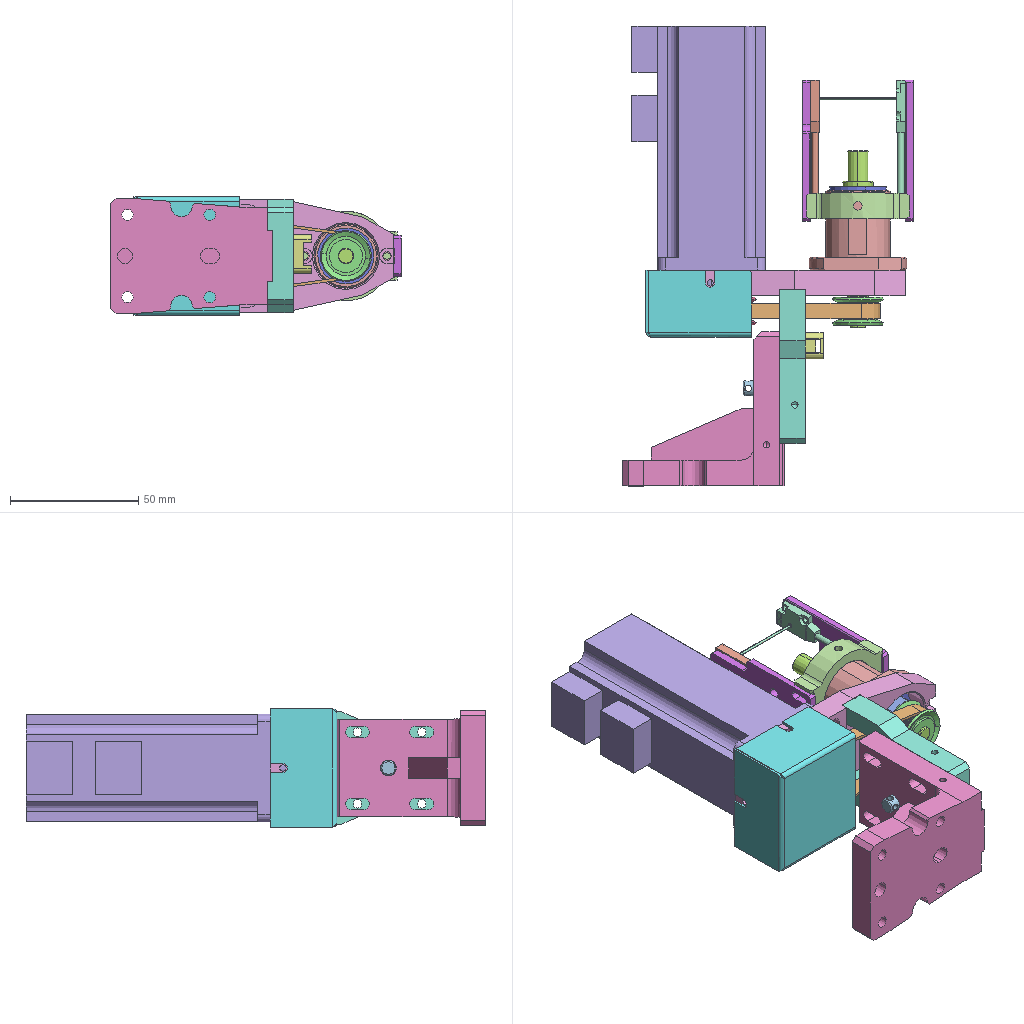Assembly | SolidWorks | 18 different items | 20 placed | box 113 x 179 x 46 mm
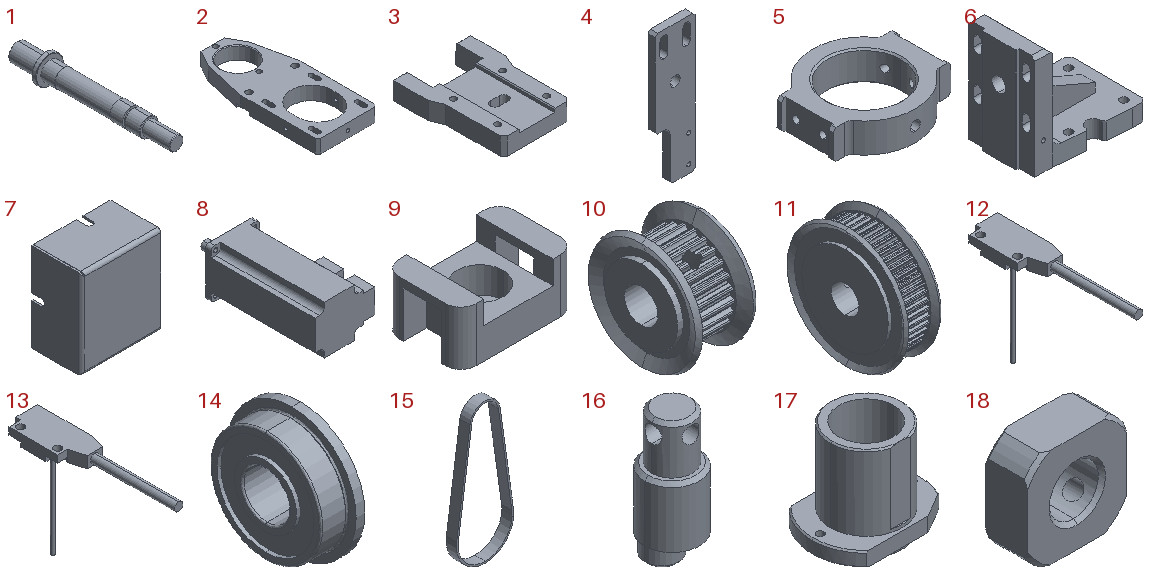Parts list (item | quantity | size | volume | features):
1 | x1 | 12 x 69 x 12 mm | 3193 mm3 | features ICE 3, Chamfer 1, Extrusion 1, RevCut 1
2 | x1 | 44 x 100 x 10 mm | 22505 mm3 | features ICE 7, HoleWzd 5, Chamfer 2, MirrorPattern 2, Cut 1, Extrusion 1, LPattern 1
3 | x1 | 44 x 60 x 10 mm | 17311 mm3 | features ICE 5, Chamfer 3, HoleWzd 3, Extrusion 1
4 | x2 | 16 x 3 x 55 mm | 2072 mm3 | features Chamfer 2, HoleWzd 2, Cut 1, Extrusion 1, Fillet 1, ICE 1
5 | x1 | 40 x 35 x 10 mm | 5332 mm3 | features ICE 3, Chamfer 2, HoleWzd 2, Extrusion 1, Fillet 1, MirrorPattern 1
6 | x1 | 62.8 x 45 x 60 mm | 46658 mm3 | features ICE 9, Chamfer 4, Cut 2, Extrusion 1, Fillet 1, HoleWzd 1, LPattern 1, MirrorPattern 1
7 | x1 | 41 x 26 x 46 mm | 4894 mm3 | features Chamfer 1, CornerFeat 1, Cut 1, EdgeFlange 1, FlatPattern 1, ICE 1, SMBaseFlange 1, SheetMetal 1
8 | x1 | 52 x 116 x 42 mm | 155076 mm3 | features ICE 7, Fillet 2, Extrusion 1
9 | x1 | 15 x 10 x 7 mm | 474.384 mm3 | features ICE 2, Extrusion 1, Fillet 1, HoleWzd 1
10 | x1 | 11 x 20 x 20 mm | 1710 mm3 | features BaseBody 1, CirPattern 1, HoleWzd 1, ICE 1
11 | x1 | 11 x 35 x 35 mm | 7284 mm3 | features BaseBody 3, CirPattern 1, HoleWzd 1
12 | x1 | 10 x 45.5 x 33.5 mm | 726.533 mm3 | features ICE 3, BaseBody 2
13 | x1 | 10 x 45.5 x 33.5 mm | 726.533 mm3 | features ICE 3, BaseBody 2
14 | x2 | 6 x 22 x 22 mm | 1366 mm3 | features BaseBody 1
15 | x1 | 33.828 x 6 x 82.868 mm | 1159 mm3 | features Extrusion 1
16 | x1 | 8 x 8 x 19.8 mm | 664.548 mm3 | features ICE 4, Chamfer 1, CirPattern 1, Extrusion 1
17 | x1 | 38 x 27 x 33 mm | 8754 mm3 | features ICE 5, Chamfer 1, Cut 1, Extrusion 1, HoleWzd 1, MirrorPattern 1
18 | x1 | 14 x 6.5 x 14 mm | 883.515 mm3 | features Chamfer 2, HoleWzd 2, ICE 2, CirPattern 1, Extrusion 1
Mates (type | each side: item.copy, entity, surface, feature):
Coincident | 3.1 face plane Boss-Extrude1 | 2.1 face plane Cut-Extrude13
Coincident | 3.1 face plane Boss-Extrude1 | 2.1 face plane Boss-Extrude1
Concentric | 1.1 face cylinder Boss-Extrude1 | 18.1 face cylinder M8x1.0 Tapped Hole1
Coincident | 2.1 face plane Boss-Extrude1 | 17.1 face plane Boss-Extrude2
Parallel | 2.1 face plane Boss-Extrude1 | 17.1 face plane Cut-Extrude1
Coincident | 2.1 face plane Boss-Extrude1 | 8.1 face plane Boss-Extrude1
Concentric | 1.1 face cylinder Boss-Extrude3 | 10.1 face cylinder Input 1
Coincident | 1.1 face plane Boss-Extrude1 | 10.1 face plane Input 1
Coincident | 10.1 face plane Input 1 | 11.1 face plane Input 1
Concentric | 8.1 face cylinder Boss-Extrude3 | 11.1 face cylinder Input 1
Concentric | 2.1 face cylinder Cut-Extrude1 | 17.1 face cylinder Boss-Extrude3
Concentric | 1.1 face cylinder Cut-Revolve1 | 17.1 face cylinder Boss-Extrude1
Concentric | 1.1 face cylinder Boss-Extrude1 | 18.1 face cylinder Boss-Extrude3
Concentric | 2.1 select_type:24 | 8.1 face cylinder Boss-Extrude3
Concentric | 15.1 face cylinder Boss-Extrude1 | 10.1 face cylinder Input 1
Concentric | 15.1 face cylinder Boss-Extrude1 | 11.1 face cylinder Input 1
DistanceDim | 11.1 face plane Input 1 | 15.1 face plane Boss-Extrude1
Parallel | 17.1 face plane Cut-Extrude1 | 2.1 face plane Boss-Extrude1
Parallel | 2.1 face plane Boss-Extrude1 | 8.1 face plane Boss-Extrude1
Coincident | 2.1 face plane Cut-Extrude13 | 3.1 face plane Boss-Extrude1
Width | 4.1 face plane Boss-Extrude1 | 4.1 face plane Boss-Extrude1 | 2.1 face plane Boss-Extrude1 | 2.1 face plane Boss-Extrude1
Coincident | 4.1 face plane Boss-Extrude1 | 4.2 face plane Boss-Extrude1
Concentric | 12.1 face cylinder Boss-Extrude1 | 13.1 face cylinder Boss-Extrude1
Coincident | 4.1 face plane Boss-Extrude1 | 12.1 face plane EX-11AD-1-solid1 | 2 times
DistanceDim | 12.1 face plane EX-11AD-1-solid1 | 4.1 face plane Boss-Extrude1
Coincident | 4.2 face plane Boss-Extrude1 | 13.1 face plane EX-11AD-1-solid1
Concentric | 4.2 face cylinder M2 Tapped Hole1 | 13.1 face cylinder EX-11AD-1-solid1
Concentric | 6.1 face cylinder Cut-Extrude9 | 16.1 face cylinder Boss-Extrude1
Coincident | 6.1 edge | 16.1 face plane Boss-Extrude1
Coincident | 1.1 face plane Boss-Extrude2 | 14.1 face plane Input 1
Coincident | 17.1 face plane Boss-Extrude1 | 14.1 face plane Input 1
Concentric | 17.1 face cylinder Boss-Extrude1 | 14.1 face cylinder Input 1
Coincident | 17.1 face plane Boss-Extrude3 | 14.2 face plane Input 1
Coincident | 18.1 face plane Boss-Extrude1 | 14.2 face plane Input 1
Concentric | 17.1 face cylinder Cut-Extrude2 | 14.2 face cylinder Input 1
Concentric | 17.1 face cylinder Boss-Extrude1 | 5.1 face cylinder Cut-Extrude1
Coincident | 4.1 face plane Boss-Extrude1 | 5.1 face plane Cut-Extrude2 | 2 times
Coincident | 4.2 face plane Boss-Extrude1 | 5.1 face plane Cut-Extrude2
DistanceDim | 4.1 face plane Boss-Extrude1 | 5.1 face plane Boss-Extrude1
DistanceDim | 17.1 face plane Boss-Extrude1 | 5.1 face plane Boss-Extrude1
DistanceDim | 1.1 face plane Boss-Extrude2 | 6.1 face plane Boss-Extrude1
Coincident | 3.1 face plane Boss-Extrude1 | 6.1 face plane Boss-Extrude1
Coincident | 3.1 face plane Cut-Extrude1 | 6.1 face plane Boss-Extrude4
Coincident | 2.1 face plane Boss-Extrude1 | 7.1 face plane Edge-Flange1 | 3 times